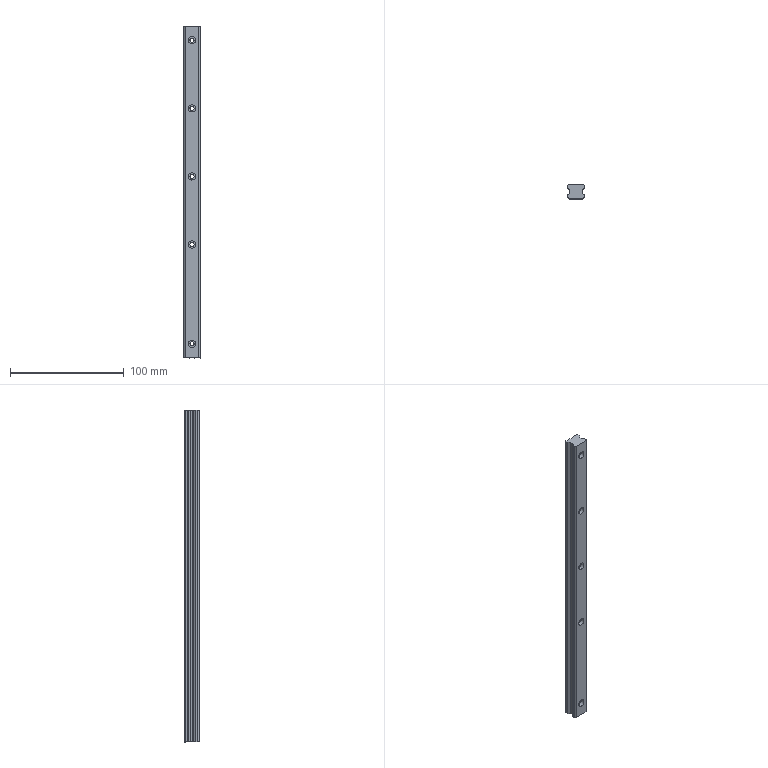Part | SolidWorks | features BaseBody 1 | 1 solid | 62 faces | box 15 x 12.5 x 292.5 mm | volume 46748 mm3 | cylinder 37 | plane 25 | commonest cylinder face diameters 0.6 x10 3.6 x10 6.5 x10 3 x5 1 x2